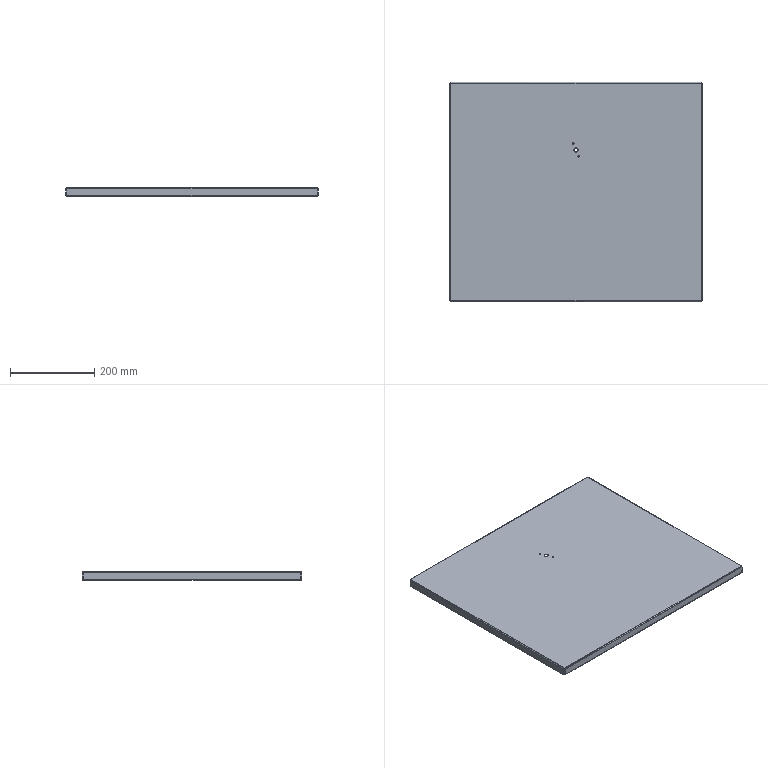Part | STEP file | Box door_default<machined> | 1 solid | 76 faces | box 600 x 522 x 20 mm | volume 571092 mm3 | plane 38 | cylinder 22 | spline 16 | commonest cylinder face diameters 1.5 x8 4.5 x8 3.2 x4 10 x2